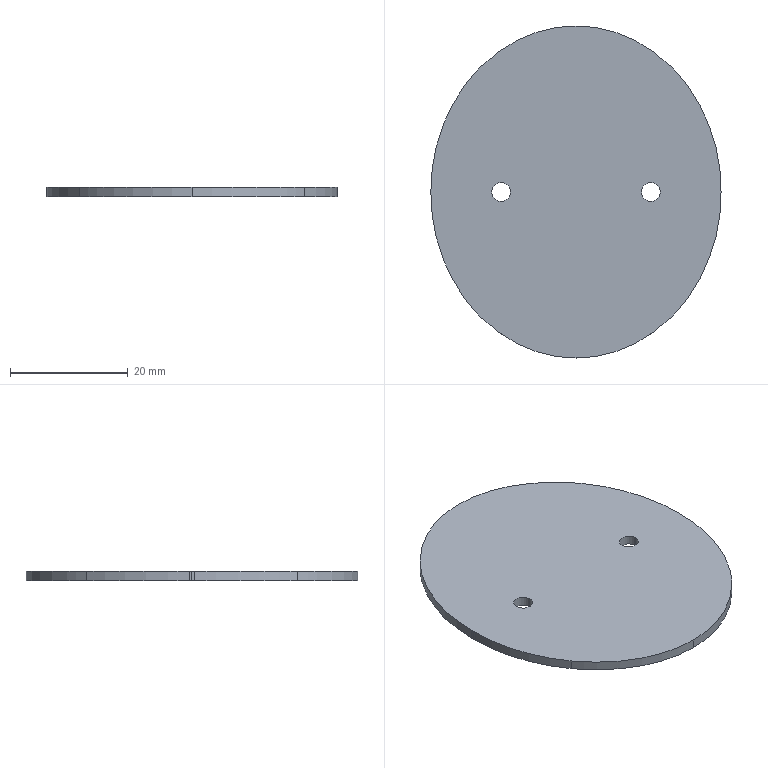Part | SolidWorks | features Extrusion 1, ICE 1 | 1 solid | 16 faces | box 49.231 x 56.342 x 1.6 mm | volume 3464 mm3 | cylinder 10 | spline 4 | plane 2 | commonest cylinder face diameters 60.146 x6 3.175 x4
STEP:
#1=CARTESIAN_POINT('',(0.4375,0.,0.));
#2=VERTEX_POINT('',#1);
#3=CARTESIAN_POINT('',(0.5625,0.,0.));
#4=VERTEX_POINT('',#3);
#5=CARTESIAN_POINT('',(0.5,0.,0.));
#6=DIRECTION('',(0.,0.,1.));
#7=DIRECTION('',(1.,0.,0.));
#8=AXIS2_PLACEMENT_3D('',#5,#6,#7);
#9=CIRCLE('',#8,0.0625);
#10=EDGE_CURVE('',#2,#4,#9,.T.);
#11=ORIENTED_EDGE('',*,*,#10,.F.);
#12=CARTESIAN_POINT('',(0.4375,0.,0.063));
#13=VERTEX_POINT('',#12);
#14=CARTESIAN_POINT('',(0.4375,0.,0.));
#15=DIRECTION('',(0.,0.,1.));
#16=VECTOR('',#15,39.37);
#17=LINE('',#14,#16);
#18=EDGE_CURVE('',#2,#13,#17,.T.);
#19=ORIENTED_EDGE('',*,*,#18,.T.);
#20=CARTESIAN_POINT('',(0.5625,0.,0.063));
#21=VERTEX_POINT('',#20);
#22=CARTESIAN_POINT('',(0.5,0.,0.063));
#23=DIRECTION('',(0.,0.,1.));
#24=DIRECTION('',(1.,0.,0.));
#25=AXIS2_PLACEMENT_3D('',#22,#23,#24);
#26=CIRCLE('',#25,0.0625);
#27=EDGE_CURVE('',#13,#21,#26,.T.);
#28=ORIENTED_EDGE('',*,*,#27,.T.);
#29=CARTESIAN_POINT('',(0.5625,0.,0.));
#30=DIRECTION('',(0.,0.,1.));
#31=VECTOR('',#30,39.37);
#32=LINE('',#29,#31);
#33=EDGE_CURVE('',#4,#21,#32,.T.);
#34=ORIENTED_EDGE('',*,*,#33,.F.);
#35=EDGE_LOOP('',(#11,#19,#28,#34));
#36=FACE_OUTER_BOUND('',#35,.T.);
#37=CARTESIAN_POINT('',(0.5,0.,0.));
#38=DIRECTION('',(0.,0.,1.));
#39=DIRECTION('',(1.,0.,0.));
#40=AXIS2_PLACEMENT_3D('',#37,#38,#39);
#41=CYLINDRICAL_SURFACE('',#40,0.0625);
#42=ADVANCED_FACE('',(#36),#41,.F.);
#43=CARTESIAN_POINT('',(-0.5625,0.,0.));
#44=VERTEX_POINT('',#43);
#45=CARTESIAN_POINT('',(-0.4375,0.,0.));
#46=VERTEX_POINT('',#45);
#47=CARTESIAN_POINT('',(-0.5,0.,0.));
#48=DIRECTION('',(0.,0.,1.));
#49=DIRECTION('',(1.,0.,0.));
#50=AXIS2_PLACEMENT_3D('',#47,#48,#49);
#51=CIRCLE('',#50,0.0625);
#52=EDGE_CURVE('',#44,#46,#51,.T.);
#53=ORIENTED_EDGE('',*,*,#52,.F.);
#54=CARTESIAN_POINT('',(-0.5625,0.,0.063));
#55=VERTEX_POINT('',#54);
#56=CARTESIAN_POINT('',(-0.5625,0.,0.));
#57=DIRECTION('',(0.,0.,1.));
#58=VECTOR('',#57,39.37);
#59=LINE('',#56,#58);
#60=EDGE_CURVE('',#44,#55,#59,.T.);
#61=ORIENTED_EDGE('',*,*,#60,.T.);
#62=CARTESIAN_POINT('',(-0.4375,0.,0.063));
#63=VERTEX_POINT('',#62);
#64=CARTESIAN_POINT('',(-0.5,0.,0.063));
#65=DIRECTION('',(0.,0.,1.));
#66=DIRECTION('',(1.,0.,0.));
#67=AXIS2_PLACEMENT_3D('',#64,#65,#66);
#68=CIRCLE('',#67,0.0625);
#69=EDGE_CURVE('',#55,#63,#68,.T.);
#70=ORIENTED_EDGE('',*,*,#69,.T.);
#71=CARTESIAN_POINT('',(-0.4375,0.,0.));
#72=DIRECTION('',(0.,0.,1.));
#73=VECTOR('',#72,39.37);
#74=LINE('',#71,#73);
#75=EDGE_CURVE('',#46,#63,#74,.T.);
#76=ORIENTED_EDGE('',*,*,#75,.F.);
#77=EDGE_LOOP('',(#53,#61,#70,#76));
#78=FACE_OUTER_BOUND('',#77,.T.);
#79=CARTESIAN_POINT('',(-0.5,0.,0.));
#80=DIRECTION('',(0.,0.,1.));
#81=DIRECTION('',(1.,0.,0.));
#82=AXIS2_PLACEMENT_3D('',#79,#80,#81);
#83=CYLINDRICAL_SURFACE('',#82,0.0625);
#84=ADVANCED_FACE('',(#78),#83,.F.);
#85=CARTESIAN_POINT('',(-0.75,-0.703,0.063));
#86=VERTEX_POINT('',#85);
#87=CARTESIAN_POINT('',(-0.9691,-0.01681,0.063));
#88=VERTEX_POINT('',#87);
#89=CARTESIAN_POINT('',(0.2149,-0.01681,0.063));
#90=DIRECTION('',(0.,0.,-1.));
#91=DIRECTION('',(1.,0.,0.));
#92=AXIS2_PLACEMENT_3D('',#89,#90,#91);
#93=CIRCLE('',#92,1.184);
#94=EDGE_CURVE('',#86,#88,#93,.T.);
#95=ORIENTED_EDGE('',*,*,#94,.T.);
#96=CARTESIAN_POINT('',(-0.9691,-0.01681,0.));
#97=VERTEX_POINT('',#96);
#98=CARTESIAN_POINT('',(-0.9691,-0.01681,0.063));
#99=DIRECTION('',(0.,0.,-1.));
#100=VECTOR('',#99,39.37);
#101=LINE('',#98,#100);
#102=EDGE_CURVE('',#88,#97,#101,.T.);
#103=ORIENTED_EDGE('',*,*,#102,.T.);
#104=CARTESIAN_POINT('',(-0.75,-0.703,0.));
#105=VERTEX_POINT('',#104);
#106=CARTESIAN_POINT('',(0.2149,-0.01681,0.));
#107=DIRECTION('',(0.,0.,-1.));
#108=DIRECTION('',(1.,0.,0.));
#109=AXIS2_PLACEMENT_3D('',#106,#107,#108);
#110=CIRCLE('',#109,1.184);
#111=EDGE_CURVE('',#105,#97,#110,.T.);
#112=ORIENTED_EDGE('',*,*,#111,.F.);
#113=CARTESIAN_POINT('',(-0.75,-0.703,0.063));
#114=DIRECTION('',(0.,0.,-1.));
#115=VECTOR('',#114,39.37);
#116=LINE('',#113,#115);
#117=EDGE_CURVE('',#86,#105,#116,.T.);
#118=ORIENTED_EDGE('',*,*,#117,.F.);
#119=EDGE_LOOP('',(#95,#103,#112,#118));
#120=FACE_OUTER_BOUND('',#119,.T.);
#121=CARTESIAN_POINT('',(0.2149,-0.01681,0.063));
#122=DIRECTION('',(0.,0.,-1.));
#123=DIRECTION('',(-1.,0.,0.));
#124=AXIS2_PLACEMENT_3D('',#121,#122,#123);
#125=CYLINDRICAL_SURFACE('',#124,1.184);
#126=ADVANCED_FACE('',(#120),#125,.T.);
#127=CARTESIAN_POINT('',(-0.9691,0.01681,0.063));
#128=VERTEX_POINT('',#127);
#129=CARTESIAN_POINT('',(-0.969,0.,0.063));
#130=VERTEX_POINT('',#129);
#131=CARTESIAN_POINT('',(0.2149,0.01681,0.063));
#132=DIRECTION('',(0.,0.,1.));
#133=DIRECTION('',(1.,0.,0.));
#134=AXIS2_PLACEMENT_3D('',#131,#132,#133);
#135=CIRCLE('',#134,1.184);
#136=EDGE_CURVE('',#128,#130,#135,.T.);
#137=ORIENTED_EDGE('',*,*,#136,.F.);
#138=CARTESIAN_POINT('',(-0.9691,0.01681,0.));
#139=VERTEX_POINT('',#138);
#140=CARTESIAN_POINT('',(-0.9691,0.01681,0.063));
#141=DIRECTION('',(0.,0.,-1.));
#142=VECTOR('',#141,39.37);
#143=LINE('',#140,#142);
#144=EDGE_CURVE('',#128,#139,#143,.T.);
#145=ORIENTED_EDGE('',*,*,#144,.T.);
#146=CARTESIAN_POINT('',(-0.969,0.,0.));
#147=VERTEX_POINT('',#146);
#148=CARTESIAN_POINT('',(0.2149,0.01681,0.));
#149=DIRECTION('',(0.,0.,1.));
#150=DIRECTION('',(1.,0.,0.));
#151=AXIS2_PLACEMENT_3D('',#148,#149,#150);
#152=CIRCLE('',#151,1.184);
#153=EDGE_CURVE('',#139,#147,#152,.T.);
#154=ORIENTED_EDGE('',*,*,#153,.T.);
#155=CARTESIAN_POINT('',(-0.969,0.,0.063));
#156=DIRECTION('',(0.,0.,-1.));
#157=VECTOR('',#156,39.37);
#158=LINE('',#155,#157);
#159=EDGE_CURVE('',#130,#147,#158,.T.);
#160=ORIENTED_EDGE('',*,*,#159,.F.);
#161=EDGE_LOOP('',(#137,#145,#154,#160));
#162=FACE_OUTER_BOUND('',#161,.T.);
#163=CARTESIAN_POINT('',(0.2149,0.01681,0.063));
#164=DIRECTION('',(0.,0.,-1.));
#165=DIRECTION('',(-1.,0.,0.));
#166=AXIS2_PLACEMENT_3D('',#163,#164,#165);
#167=CYLINDRICAL_SURFACE('',#166,1.184);
#168=ADVANCED_FACE('',(#162),#167,.T.);
#169=CARTESIAN_POINT('',(0.,-1.109,0.));
#170=VERTEX_POINT('',#169);
#171=CARTESIAN_POINT('',(0.,-1.109,0.));
#172=CARTESIAN_POINT('',(-0.2983,-1.114,0.));
#173=CARTESIAN_POINT('',(-0.5795,-0.9413,0.));
#174=CARTESIAN_POINT('',(-0.75,-0.703,0.));
#175=B_SPLINE_CURVE_WITH_KNOTS('',3,(#171,#172,#173,#174),.UNSPECIFIED.,.F.,.F.,(4,4),(0.,1.),.UNSPECIFIED.);
#176=EDGE_CURVE('',#170,#105,#175,.T.);
#177=ORIENTED_EDGE('',*,*,#176,.F.);
#178=CARTESIAN_POINT('',(0.,-1.109,0.063));
#179=VERTEX_POINT('',#178);
#180=CARTESIAN_POINT('',(0.,-1.109,0.063));
#181=DIRECTION('',(0.,0.,-1.));
#182=VECTOR('',#181,39.37);
#183=LINE('',#180,#182);
#184=EDGE_CURVE('',#179,#170,#183,.T.);
#185=ORIENTED_EDGE('',*,*,#184,.F.);
#186=CARTESIAN_POINT('',(0.,-1.109,0.063));
#187=CARTESIAN_POINT('',(-0.2983,-1.114,0.063));
#188=CARTESIAN_POINT('',(-0.5795,-0.9413,0.063));
#189=CARTESIAN_POINT('',(-0.75,-0.703,0.063));
#190=B_SPLINE_CURVE_WITH_KNOTS('',3,(#186,#187,#188,#189),.UNSPECIFIED.,.F.,.F.,(4,4),(0.,1.),.UNSPECIFIED.);
#191=EDGE_CURVE('',#179,#86,#190,.T.);
#192=ORIENTED_EDGE('',*,*,#191,.T.);
#193=ORIENTED_EDGE('',*,*,#117,.T.);
#194=EDGE_LOOP('',(#177,#185,#192,#193));
#195=FACE_OUTER_BOUND('',#194,.T.);
#196=CARTESIAN_POINT('',(0.,-1.109,0.063));
#197=CARTESIAN_POINT('',(0.,-1.109,0.));
#198=CARTESIAN_POINT('',(-0.2983,-1.114,0.063));
#199=CARTESIAN_POINT('',(-0.2983,-1.114,0.));
#200=CARTESIAN_POINT('',(-0.5795,-0.9413,0.063));
#201=CARTESIAN_POINT('',(-0.5795,-0.9413,0.));
#202=CARTESIAN_POINT('',(-0.75,-0.703,0.063));
#203=CARTESIAN_POINT('',(-0.75,-0.703,0.));
#204=B_SPLINE_SURFACE_WITH_KNOTS('',3,1,((#196,#197),(#198,#199),(#200,#201),(#202,#203)),.UNSPECIFIED.,.F.,.F.,.F.,(4,4),(2,2),(0.,1.),(0.,1.),.UNSPECIFIED.);
#205=ADVANCED_FACE('',(#195),#204,.T.);
#206=CARTESIAN_POINT('',(0.75,-0.703,0.));
#207=VERTEX_POINT('',#206);
#208=CARTESIAN_POINT('',(0.,-1.109,0.));
#209=CARTESIAN_POINT('',(0.2983,-1.114,0.));
#210=CARTESIAN_POINT('',(0.5795,-0.9413,0.));
#211=CARTESIAN_POINT('',(0.75,-0.703,0.));
#212=B_SPLINE_CURVE_WITH_KNOTS('',3,(#208,#209,#210,#211),.UNSPECIFIED.,.F.,.F.,(4,4),(0.,1.),.UNSPECIFIED.);
#213=EDGE_CURVE('',#170,#207,#212,.T.);
#214=ORIENTED_EDGE('',*,*,#213,.T.);
#215=CARTESIAN_POINT('',(0.75,-0.703,0.063));
#216=VERTEX_POINT('',#215);
#217=CARTESIAN_POINT('',(0.75,-0.703,0.063));
#218=DIRECTION('',(0.,0.,-1.));
#219=VECTOR('',#218,39.37);
#220=LINE('',#217,#219);
#221=EDGE_CURVE('',#216,#207,#220,.T.);
#222=ORIENTED_EDGE('',*,*,#221,.F.);
#223=CARTESIAN_POINT('',(0.,-1.109,0.063));
#224=CARTESIAN_POINT('',(0.2983,-1.114,0.063));
#225=CARTESIAN_POINT('',(0.5795,-0.9413,0.063));
#226=CARTESIAN_POINT('',(0.75,-0.703,0.063));
#227=B_SPLINE_CURVE_WITH_KNOTS('',3,(#223,#224,#225,#226),.UNSPECIFIED.,.F.,.F.,(4,4),(0.,1.),.UNSPECIFIED.);
#228=EDGE_CURVE('',#179,#216,#227,.T.);
#229=ORIENTED_EDGE('',*,*,#228,.F.);
#230=ORIENTED_EDGE('',*,*,#184,.T.);
#231=EDGE_LOOP('',(#214,#222,#229,#230));
#232=FACE_OUTER_BOUND('',#231,.T.);
#233=CARTESIAN_POINT('',(0.,-1.109,0.063));
#234=CARTESIAN_POINT('',(0.,-1.109,0.));
#235=CARTESIAN_POINT('',(0.2983,-1.114,0.063));
#236=CARTESIAN_POINT('',(0.2983,-1.114,0.));
#237=CARTESIAN_POINT('',(0.5795,-0.9413,0.063));
#238=CARTESIAN_POINT('',(0.5795,-0.9413,0.));
#239=CARTESIAN_POINT('',(0.75,-0.703,0.063));
#240=CARTESIAN_POINT('',(0.75,-0.703,0.));
#241=B_SPLINE_SURFACE_WITH_KNOTS('',3,1,((#233,#234),(#235,#236),(#237,#238),(#239,#240)),.UNSPECIFIED.,.F.,.F.,.F.,(4,4),(2,2),(0.,1.),(0.,1.),.UNSPECIFIED.);
#242=ADVANCED_FACE('',(#232),#241,.F.);
#243=CARTESIAN_POINT('',(0.969,0.,0.));
#244=VERTEX_POINT('',#243);
#245=CARTESIAN_POINT('',(-0.2149,-0.01681,0.));
#246=DIRECTION('',(0.,0.,1.));
#247=DIRECTION('',(1.,0.,0.));
#248=AXIS2_PLACEMENT_3D('',#245,#246,#247);
#249=CIRCLE('',#248,1.184);
#250=EDGE_CURVE('',#207,#244,#249,.T.);
#251=ORIENTED_EDGE('',*,*,#250,.T.);
#252=CARTESIAN_POINT('',(0.969,0.,0.063));
#253=VERTEX_POINT('',#252);
#254=CARTESIAN_POINT('',(0.969,0.,0.063));
#255=DIRECTION('',(0.,0.,-1.));
#256=VECTOR('',#255,39.37);
#257=LINE('',#254,#256);
#258=EDGE_CURVE('',#253,#244,#257,.T.);
#259=ORIENTED_EDGE('',*,*,#258,.F.);
#260=CARTESIAN_POINT('',(-0.2149,-0.01681,0.063));
#261=DIRECTION('',(0.,0.,1.));
#262=DIRECTION('',(1.,0.,0.));
#263=AXIS2_PLACEMENT_3D('',#260,#261,#262);
#264=CIRCLE('',#263,1.184);
#265=EDGE_CURVE('',#216,#253,#264,.T.);
#266=ORIENTED_EDGE('',*,*,#265,.F.);
#267=ORIENTED_EDGE('',*,*,#221,.T.);
#268=EDGE_LOOP('',(#251,#259,#266,#267));
#269=FACE_OUTER_BOUND('',#268,.T.);
#270=CARTESIAN_POINT('',(-0.2149,-0.01681,0.063));
#271=DIRECTION('',(0.,0.,-1.));
#272=DIRECTION('',(-1.,0.,0.));
#273=AXIS2_PLACEMENT_3D('',#270,#271,#272);
#274=CYLINDRICAL_SURFACE('',#273,1.184);
#275=ADVANCED_FACE('',(#269),#274,.T.);
#276=CARTESIAN_POINT('',(0.75,0.703,0.));
#277=VERTEX_POINT('',#276);
#278=CARTESIAN_POINT('',(-0.2149,0.01681,0.));
#279=DIRECTION('',(0.,0.,-1.));
#280=DIRECTION('',(1.,0.,0.));
#281=AXIS2_PLACEMENT_3D('',#278,#279,#280);
#282=CIRCLE('',#281,1.184);
#283=EDGE_CURVE('',#277,#244,#282,.T.);
#284=ORIENTED_EDGE('',*,*,#283,.F.);
#285=CARTESIAN_POINT('',(0.75,0.703,0.063));
#286=VERTEX_POINT('',#285);
#287=CARTESIAN_POINT('',(0.75,0.703,0.063));
#288=DIRECTION('',(0.,0.,-1.));
#289=VECTOR('',#288,39.37);
#290=LINE('',#287,#289);
#291=EDGE_CURVE('',#286,#277,#290,.T.);
#292=ORIENTED_EDGE('',*,*,#291,.F.);
#293=CARTESIAN_POINT('',(-0.2149,0.01681,0.063));
#294=DIRECTION('',(0.,0.,-1.));
#295=DIRECTION('',(1.,0.,0.));
#296=AXIS2_PLACEMENT_3D('',#293,#294,#295);
#297=CIRCLE('',#296,1.184);
#298=EDGE_CURVE('',#286,#253,#297,.T.);
#299=ORIENTED_EDGE('',*,*,#298,.T.);
#300=ORIENTED_EDGE('',*,*,#258,.T.);
#301=EDGE_LOOP('',(#284,#292,#299,#300));
#302=FACE_OUTER_BOUND('',#301,.T.);
#303=CARTESIAN_POINT('',(-0.2149,0.01681,0.063));
#304=DIRECTION('',(0.,0.,-1.));
#305=DIRECTION('',(-1.,0.,0.));
#306=AXIS2_PLACEMENT_3D('',#303,#304,#305);
#307=CYLINDRICAL_SURFACE('',#306,1.184);
#308=ADVANCED_FACE('',(#302),#307,.T.);
#309=CARTESIAN_POINT('',(0.,1.109,0.));
#310=VERTEX_POINT('',#309);
#311=CARTESIAN_POINT('',(0.,1.109,0.));
#312=CARTESIAN_POINT('',(0.2983,1.114,0.));
#313=CARTESIAN_POINT('',(0.5795,0.9413,0.));
#314=CARTESIAN_POINT('',(0.75,0.703,0.));
#315=B_SPLINE_CURVE_WITH_KNOTS('',3,(#311,#312,#313,#314),.UNSPECIFIED.,.F.,.F.,(4,4),(0.,1.),.UNSPECIFIED.);
#316=EDGE_CURVE('',#310,#277,#315,.T.);
#317=ORIENTED_EDGE('',*,*,#316,.F.);
#318=CARTESIAN_POINT('',(0.,1.109,0.063));
#319=VERTEX_POINT('',#318);
#320=CARTESIAN_POINT('',(0.,1.109,0.063));
#321=DIRECTION('',(0.,0.,-1.));
#322=VECTOR('',#321,39.37);
#323=LINE('',#320,#322);
#324=EDGE_CURVE('',#319,#310,#323,.T.);
#325=ORIENTED_EDGE('',*,*,#324,.F.);
#326=CARTESIAN_POINT('',(0.,1.109,0.063));
#327=CARTESIAN_POINT('',(0.2983,1.114,0.063));
#328=CARTESIAN_POINT('',(0.5795,0.9413,0.063));
#329=CARTESIAN_POINT('',(0.75,0.703,0.063));
#330=B_SPLINE_CURVE_WITH_KNOTS('',3,(#326,#327,#328,#329),.UNSPECIFIED.,.F.,.F.,(4,4),(0.,1.),.UNSPECIFIED.);
#331=EDGE_CURVE('',#319,#286,#330,.T.);
#332=ORIENTED_EDGE('',*,*,#331,.T.);
#333=ORIENTED_EDGE('',*,*,#291,.T.);
#334=EDGE_LOOP('',(#317,#325,#332,#333));
#335=FACE_OUTER_BOUND('',#334,.T.);
#336=CARTESIAN_POINT('',(0.,1.109,0.063));
#337=CARTESIAN_POINT('',(0.,1.109,0.));
#338=CARTESIAN_POINT('',(0.2983,1.114,0.063));
#339=CARTESIAN_POINT('',(0.2983,1.114,0.));
#340=CARTESIAN_POINT('',(0.5795,0.9413,0.063));
#341=CARTESIAN_POINT('',(0.5795,0.9413,0.));
#342=CARTESIAN_POINT('',(0.75,0.703,0.063));
#343=CARTESIAN_POINT('',(0.75,0.703,0.));
#344=B_SPLINE_SURFACE_WITH_KNOTS('',3,1,((#336,#337),(#338,#339),(#340,#341),(#342,#343)),.UNSPECIFIED.,.F.,.F.,.F.,(4,4),(2,2),(0.,1.),(0.,1.),.UNSPECIFIED.);
#345=ADVANCED_FACE('',(#335),#344,.T.);
#346=CARTESIAN_POINT('',(-0.75,0.703,0.));
#347=VERTEX_POINT('',#346);
#348=CARTESIAN_POINT('',(0.,1.109,0.));
#349=CARTESIAN_POINT('',(-0.2983,1.114,0.));
#350=CARTESIAN_POINT('',(-0.5795,0.9413,0.));
#351=CARTESIAN_POINT('',(-0.75,0.703,0.));
#352=B_SPLINE_CURVE_WITH_KNOTS('',3,(#348,#349,#350,#351),.UNSPECIFIED.,.F.,.F.,(4,4),(0.,1.),.UNSPECIFIED.);
#353=EDGE_CURVE('',#310,#347,#352,.T.);
#354=ORIENTED_EDGE('',*,*,#353,.T.);
#355=CARTESIAN_POINT('',(-0.75,0.703,0.063));
#356=VERTEX_POINT('',#355);
#357=CARTESIAN_POINT('',(-0.75,0.703,0.063));
#358=DIRECTION('',(0.,0.,-1.));
#359=VECTOR('',#358,39.37);
#360=LINE('',#357,#359);
#361=EDGE_CURVE('',#356,#347,#360,.T.);
#362=ORIENTED_EDGE('',*,*,#361,.F.);
#363=CARTESIAN_POINT('',(0.,1.109,0.063));
#364=CARTESIAN_POINT('',(-0.2983,1.114,0.063));
#365=CARTESIAN_POINT('',(-0.5795,0.9413,0.063));
#366=CARTESIAN_POINT('',(-0.75,0.703,0.063));
#367=B_SPLINE_CURVE_WITH_KNOTS('',3,(#363,#364,#365,#366),.UNSPECIFIED.,.F.,.F.,(4,4),(0.,1.),.UNSPECIFIED.);
#368=EDGE_CURVE('',#319,#356,#367,.T.);
#369=ORIENTED_EDGE('',*,*,#368,.F.);
#370=ORIENTED_EDGE('',*,*,#324,.T.);
#371=EDGE_LOOP('',(#354,#362,#369,#370));
#372=FACE_OUTER_BOUND('',#371,.T.);
#373=CARTESIAN_POINT('',(0.,1.109,0.063));
#374=CARTESIAN_POINT('',(0.,1.109,0.));
#375=CARTESIAN_POINT('',(-0.2983,1.114,0.063));
#376=CARTESIAN_POINT('',(-0.2983,1.114,0.));
#377=CARTESIAN_POINT('',(-0.5795,0.9413,0.063));
#378=CARTESIAN_POINT('',(-0.5795,0.9413,0.));
#379=CARTESIAN_POINT('',(-0.75,0.703,0.063));
#380=CARTESIAN_POINT('',(-0.75,0.703,0.));
#381=B_SPLINE_SURFACE_WITH_KNOTS('',3,1,((#373,#374),(#375,#376),(#377,#378),(#379,#380)),.UNSPECIFIED.,.F.,.F.,.F.,(4,4),(2,2),(0.,1.),(0.,1.),.UNSPECIFIED.);
#382=ADVANCED_FACE('',(#372),#381,.F.);
#383=ORIENTED_EDGE('',*,*,#144,.F.);
#384=CARTESIAN_POINT('',(0.2149,0.01681,0.063));
#385=DIRECTION('',(0.,0.,1.));
#386=DIRECTION('',(1.,0.,0.));
#387=AXIS2_PLACEMENT_3D('',#384,#385,#386);
#388=CIRCLE('',#387,1.184);
#389=EDGE_CURVE('',#356,#128,#388,.T.);
#390=ORIENTED_EDGE('',*,*,#389,.F.);
#391=ORIENTED_EDGE('',*,*,#361,.T.);
#392=CARTESIAN_POINT('',(0.2149,0.01681,0.));
#393=DIRECTION('',(0.,0.,1.));
#394=DIRECTION('',(1.,0.,0.));
#395=AXIS2_PLACEMENT_3D('',#392,#393,#394);
#396=CIRCLE('',#395,1.184);
#397=EDGE_CURVE('',#347,#139,#396,.T.);
#398=ORIENTED_EDGE('',*,*,#397,.T.);
#399=EDGE_LOOP('',(#383,#390,#391,#398));
#400=FACE_OUTER_BOUND('',#399,.T.);
#401=CARTESIAN_POINT('',(0.2149,0.01681,0.063));
#402=DIRECTION('',(0.,0.,-1.));
#403=DIRECTION('',(-1.,0.,0.));
#404=AXIS2_PLACEMENT_3D('',#401,#402,#403);
#405=CYLINDRICAL_SURFACE('',#404,1.184);
#406=ADVANCED_FACE('',(#400),#405,.T.);
#407=ORIENTED_EDGE('',*,*,#102,.F.);
#408=CARTESIAN_POINT('',(0.2149,-0.01681,0.063));
#409=DIRECTION('',(0.,0.,-1.));
#410=DIRECTION('',(1.,0.,0.));
#411=AXIS2_PLACEMENT_3D('',#408,#409,#410);
#412=CIRCLE('',#411,1.184);
#413=EDGE_CURVE('',#88,#130,#412,.T.);
#414=ORIENTED_EDGE('',*,*,#413,.T.);
#415=ORIENTED_EDGE('',*,*,#159,.T.);
#416=CARTESIAN_POINT('',(0.2149,-0.01681,0.));
#417=DIRECTION('',(0.,0.,-1.));
#418=DIRECTION('',(1.,0.,0.));
#419=AXIS2_PLACEMENT_3D('',#416,#417,#418);
#420=CIRCLE('',#419,1.184);
#421=EDGE_CURVE('',#97,#147,#420,.T.);
#422=ORIENTED_EDGE('',*,*,#421,.F.);
#423=EDGE_LOOP('',(#407,#414,#415,#422));
#424=FACE_OUTER_BOUND('',#423,.T.);
#425=CARTESIAN_POINT('',(0.2149,-0.01681,0.063));
#426=DIRECTION('',(0.,0.,-1.));
#427=DIRECTION('',(-1.,0.,0.));
#428=AXIS2_PLACEMENT_3D('',#425,#426,#427);
#429=CYLINDRICAL_SURFACE('',#428,1.184);
#430=ADVANCED_FACE('',(#424),#429,.T.);
#431=CARTESIAN_POINT('',(0.5,0.,0.063));
#432=DIRECTION('',(0.,0.,1.));
#433=DIRECTION('',(1.,0.,0.));
#434=AXIS2_PLACEMENT_3D('',#431,#432,#433);
#435=CIRCLE('',#434,0.0625);
#436=EDGE_CURVE('',#21,#13,#435,.T.);
#437=ORIENTED_EDGE('',*,*,#436,.F.);
#438=ORIENTED_EDGE('',*,*,#27,.F.);
#439=EDGE_LOOP('',(#437,#438));
#440=FACE_BOUND('',#439,.T.);
#441=CARTESIAN_POINT('',(-0.5,0.,0.063));
#442=DIRECTION('',(0.,0.,1.));
#443=DIRECTION('',(1.,0.,0.));
#444=AXIS2_PLACEMENT_3D('',#441,#442,#443);
#445=CIRCLE('',#444,0.0625);
#446=EDGE_CURVE('',#63,#55,#445,.T.);
#447=ORIENTED_EDGE('',*,*,#446,.F.);
#448=ORIENTED_EDGE('',*,*,#69,.F.);
#449=EDGE_LOOP('',(#447,#448));
#450=FACE_BOUND('',#449,.T.);
#451=ORIENTED_EDGE('',*,*,#191,.F.);
#452=ORIENTED_EDGE('',*,*,#228,.T.);
#453=ORIENTED_EDGE('',*,*,#265,.T.);
#454=ORIENTED_EDGE('',*,*,#298,.F.);
#455=ORIENTED_EDGE('',*,*,#331,.F.);
#456=ORIENTED_EDGE('',*,*,#368,.T.);
#457=ORIENTED_EDGE('',*,*,#389,.T.);
#458=ORIENTED_EDGE('',*,*,#136,.T.);
#459=ORIENTED_EDGE('',*,*,#413,.F.);
#460=ORIENTED_EDGE('',*,*,#94,.F.);
#461=EDGE_LOOP('',(#451,#452,#453,#454,#455,#456,#457,#458,#459,#460));
#462=FACE_OUTER_BOUND('',#461,.T.);
#463=CARTESIAN_POINT('',(0.,0.,0.063));
#464=DIRECTION('',(0.,0.,1.));
#465=DIRECTION('',(1.,0.,0.));
#466=AXIS2_PLACEMENT_3D('',#463,#464,#465);
#467=PLANE('',#466);
#468=ADVANCED_FACE('',(#440,#450,#462),#467,.T.);
#469=CARTESIAN_POINT('',(0.5,0.,0.));
#470=DIRECTION('',(0.,0.,1.));
#471=DIRECTION('',(1.,0.,0.));
#472=AXIS2_PLACEMENT_3D('',#469,#470,#471);
#473=CIRCLE('',#472,0.0625);
#474=EDGE_CURVE('',#4,#2,#473,.T.);
#475=ORIENTED_EDGE('',*,*,#474,.T.);
#476=ORIENTED_EDGE('',*,*,#10,.T.);
#477=EDGE_LOOP('',(#475,#476));
#478=FACE_BOUND('',#477,.T.);
#479=CARTESIAN_POINT('',(-0.5,0.,0.));
#480=DIRECTION('',(0.,0.,1.));
#481=DIRECTION('',(1.,0.,0.));
#482=AXIS2_PLACEMENT_3D('',#479,#480,#481);
#483=CIRCLE('',#482,0.0625);
#484=EDGE_CURVE('',#46,#44,#483,.T.);
#485=ORIENTED_EDGE('',*,*,#484,.T.);
#486=ORIENTED_EDGE('',*,*,#52,.T.);
#487=EDGE_LOOP('',(#485,#486));
#488=FACE_BOUND('',#487,.T.);
#489=ORIENTED_EDGE('',*,*,#176,.T.);
#490=ORIENTED_EDGE('',*,*,#111,.T.);
#491=ORIENTED_EDGE('',*,*,#421,.T.);
#492=ORIENTED_EDGE('',*,*,#153,.F.);
#493=ORIENTED_EDGE('',*,*,#397,.F.);
#494=ORIENTED_EDGE('',*,*,#353,.F.);
#495=ORIENTED_EDGE('',*,*,#316,.T.);
#496=ORIENTED_EDGE('',*,*,#283,.T.);
#497=ORIENTED_EDGE('',*,*,#250,.F.);
#498=ORIENTED_EDGE('',*,*,#213,.F.);
#499=EDGE_LOOP('',(#489,#490,#491,#492,#493,#494,#495,#496,#497,#498));
#500=FACE_OUTER_BOUND('',#499,.T.);
#501=CARTESIAN_POINT('',(0.,0.,0.));
#502=DIRECTION('',(0.,0.,1.));
#503=DIRECTION('',(1.,0.,0.));
#504=AXIS2_PLACEMENT_3D('',#501,#502,#503);
#505=PLANE('',#504);
#506=ADVANCED_FACE('',(#478,#488,#500),#505,.F.);
#507=ORIENTED_EDGE('',*,*,#60,.F.);
#508=ORIENTED_EDGE('',*,*,#484,.F.);
#509=ORIENTED_EDGE('',*,*,#75,.T.);
#510=ORIENTED_EDGE('',*,*,#446,.T.);
#511=EDGE_LOOP('',(#507,#508,#509,#510));
#512=FACE_OUTER_BOUND('',#511,.T.);
#513=CARTESIAN_POINT('',(-0.5,0.,0.));
#514=DIRECTION('',(0.,0.,1.));
#515=DIRECTION('',(1.,0.,0.));
#516=AXIS2_PLACEMENT_3D('',#513,#514,#515);
#517=CYLINDRICAL_SURFACE('',#516,0.0625);
#518=ADVANCED_FACE('',(#512),#517,.F.);
#519=ORIENTED_EDGE('',*,*,#18,.F.);
#520=ORIENTED_EDGE('',*,*,#474,.F.);
#521=ORIENTED_EDGE('',*,*,#33,.T.);
#522=ORIENTED_EDGE('',*,*,#436,.T.);
#523=EDGE_LOOP('',(#519,#520,#521,#522));
#524=FACE_OUTER_BOUND('',#523,.T.);
#525=CARTESIAN_POINT('',(0.5,0.,0.));
#526=DIRECTION('',(0.,0.,1.));
#527=DIRECTION('',(1.,0.,0.));
#528=AXIS2_PLACEMENT_3D('',#525,#526,#527);
#529=CYLINDRICAL_SURFACE('',#528,0.0625);
#530=ADVANCED_FACE('',(#524),#529,.F.);
#531=CLOSED_SHELL('',(#42,#84,#126,#168,#205,#242,#275,#308,#345,#382,#406,#430,#468,#506,#518,#530));
#532=MANIFOLD_SOLID_BREP('',#531);
#533=CARTESIAN_POINT('',(0.,0.,0.));
#534=DIRECTION('',(0.,0.,1.));
#535=DIRECTION('',(1.,0.,0.));
#536=AXIS2_PLACEMENT_3D('',#533,#534,#535);
#537=(LENGTH_UNIT()NAMED_UNIT(*)SI_UNIT($,.METRE.));
#538=LENGTH_MEASURE_WITH_UNIT(LENGTH_MEASURE(0.0254),#537);
#539=DIMENSIONAL_EXPONENTS(1.,0.,0.,0.,0.,0.,0.);
#540=(CONVERSION_BASED_UNIT('INCH',#538)LENGTH_UNIT()NAMED_UNIT(#539));
#541=UNCERTAINTY_MEASURE_WITH_UNIT(LENGTH_MEASURE(0.00001),#540,'','');
#542=(NAMED_UNIT(*)PLANE_ANGLE_UNIT()SI_UNIT($,.RADIAN.));
#543=(NAMED_UNIT(*)SI_UNIT($,.STERADIAN.)SOLID_ANGLE_UNIT());
#544=(GEOMETRIC_REPRESENTATION_CONTEXT(3)GLOBAL_UNCERTAINTY_ASSIGNED_CONTEXT((#541))GLOBAL_UNIT_ASSIGNED_CONTEXT((#540,#542,#543))REPRESENTATION_CONTEXT('',''));
#545=ADVANCED_BREP_SHAPE_REPRESENTATION('',(#532,#536),#544);